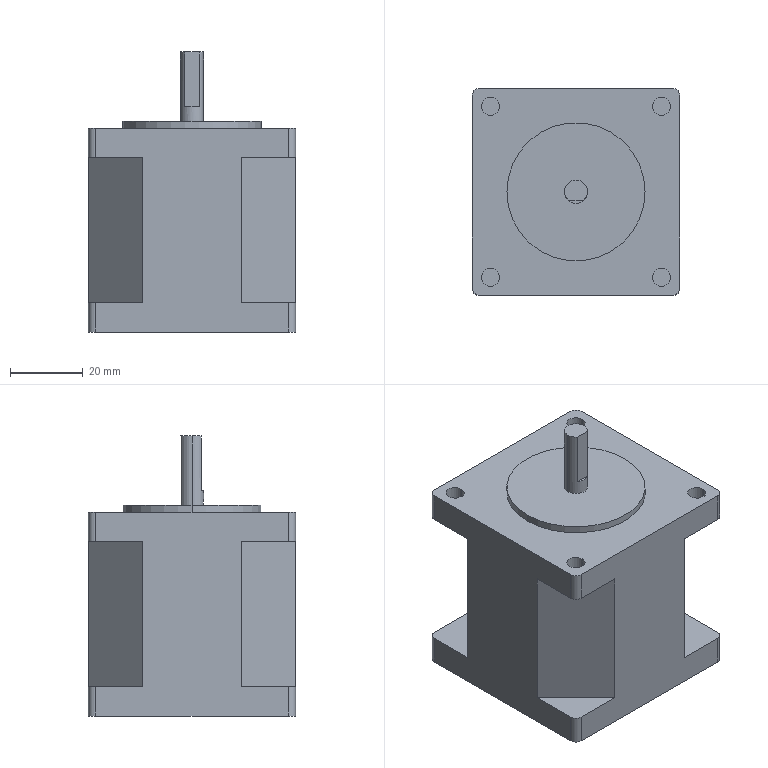Part | SolidWorks | features ICE 5, CirPattern 1, Extrusion 1, Fillet 1 | 1 solid | 42 faces | box 57 x 57 x 77 mm | volume 166104 mm3 | plane 22 | cylinder 20 | commonest cylinder face diameters 4 x8 5 x8 6.35 x2 38 x2
STEP:
#1=CARTESIAN_POINT('',(-26.,23.5,48.));
#2=VERTEX_POINT('',#1);
#3=CARTESIAN_POINT('',(-21.,23.5,48.));
#4=VERTEX_POINT('',#3);
#5=CARTESIAN_POINT('',(-23.5,23.5,48.));
#6=DIRECTION('',(0.,0.,1.));
#7=DIRECTION('',(-1.,0.,0.));
#8=AXIS2_PLACEMENT_3D('',#5,#6,#7);
#9=CIRCLE('',#8,2.5);
#10=EDGE_CURVE('',#2,#4,#9,.T.);
#11=ORIENTED_EDGE('',*,*,#10,.F.);
#12=CARTESIAN_POINT('',(-26.,23.5,56.));
#13=VERTEX_POINT('',#12);
#14=CARTESIAN_POINT('',(-26.,23.5,40.929));
#15=DIRECTION('',(0.,0.,1.));
#16=VECTOR('',#15,1000.);
#17=LINE('',#14,#16);
#18=EDGE_CURVE('',#2,#13,#17,.T.);
#19=ORIENTED_EDGE('',*,*,#18,.T.);
#20=CARTESIAN_POINT('',(-21.,23.5,56.));
#21=VERTEX_POINT('',#20);
#22=CARTESIAN_POINT('',(-23.5,23.5,56.));
#23=DIRECTION('',(0.,0.,1.));
#24=DIRECTION('',(0.,1.,0.));
#25=AXIS2_PLACEMENT_3D('',#22,#23,#24);
#26=CIRCLE('',#25,2.5);
#27=EDGE_CURVE('',#13,#21,#26,.T.);
#28=ORIENTED_EDGE('',*,*,#27,.T.);
#29=CARTESIAN_POINT('',(-21.,23.5,40.929));
#30=DIRECTION('',(0.,0.,1.));
#31=VECTOR('',#30,1000.);
#32=LINE('',#29,#31);
#33=EDGE_CURVE('',#4,#21,#32,.T.);
#34=ORIENTED_EDGE('',*,*,#33,.F.);
#35=EDGE_LOOP('',(#11,#19,#28,#34));
#36=FACE_OUTER_BOUND('',#35,.T.);
#37=CARTESIAN_POINT('',(-23.5,23.5,40.929));
#38=DIRECTION('',(0.,0.,1.));
#39=DIRECTION('',(1.,0.,0.));
#40=AXIS2_PLACEMENT_3D('',#37,#38,#39);
#41=CYLINDRICAL_SURFACE('',#40,2.5);
#42=ADVANCED_FACE('',(#36),#41,.F.);
#43=CARTESIAN_POINT('',(-26.,-23.5,48.));
#44=VERTEX_POINT('',#43);
#45=CARTESIAN_POINT('',(-21.,-23.5,48.));
#46=VERTEX_POINT('',#45);
#47=CARTESIAN_POINT('',(-23.5,-23.5,48.));
#48=DIRECTION('',(0.,0.,1.));
#49=DIRECTION('',(-1.,0.,0.));
#50=AXIS2_PLACEMENT_3D('',#47,#48,#49);
#51=CIRCLE('',#50,2.5);
#52=EDGE_CURVE('',#44,#46,#51,.T.);
#53=ORIENTED_EDGE('',*,*,#52,.F.);
#54=CARTESIAN_POINT('',(-26.,-23.5,56.));
#55=VERTEX_POINT('',#54);
#56=CARTESIAN_POINT('',(-26.,-23.5,40.929));
#57=DIRECTION('',(0.,0.,1.));
#58=VECTOR('',#57,1000.);
#59=LINE('',#56,#58);
#60=EDGE_CURVE('',#44,#55,#59,.T.);
#61=ORIENTED_EDGE('',*,*,#60,.T.);
#62=CARTESIAN_POINT('',(-21.,-23.5,56.));
#63=VERTEX_POINT('',#62);
#64=CARTESIAN_POINT('',(-23.5,-23.5,56.));
#65=DIRECTION('',(0.,0.,1.));
#66=DIRECTION('',(-1.,0.,0.));
#67=AXIS2_PLACEMENT_3D('',#64,#65,#66);
#68=CIRCLE('',#67,2.5);
#69=EDGE_CURVE('',#55,#63,#68,.T.);
#70=ORIENTED_EDGE('',*,*,#69,.T.);
#71=CARTESIAN_POINT('',(-21.,-23.5,40.929));
#72=DIRECTION('',(0.,0.,1.));
#73=VECTOR('',#72,1000.);
#74=LINE('',#71,#73);
#75=EDGE_CURVE('',#46,#63,#74,.T.);
#76=ORIENTED_EDGE('',*,*,#75,.F.);
#77=EDGE_LOOP('',(#53,#61,#70,#76));
#78=FACE_OUTER_BOUND('',#77,.T.);
#79=CARTESIAN_POINT('',(-23.5,-23.5,40.929));
#80=DIRECTION('',(0.,0.,1.));
#81=DIRECTION('',(1.,0.,0.));
#82=AXIS2_PLACEMENT_3D('',#79,#80,#81);
#83=CYLINDRICAL_SURFACE('',#82,2.5);
#84=ADVANCED_FACE('',(#78),#83,.F.);
#85=CARTESIAN_POINT('',(21.,-23.5,48.));
#86=VERTEX_POINT('',#85);
#87=CARTESIAN_POINT('',(26.,-23.5,48.));
#88=VERTEX_POINT('',#87);
#89=CARTESIAN_POINT('',(23.5,-23.5,48.));
#90=DIRECTION('',(0.,0.,1.));
#91=DIRECTION('',(-1.,0.,0.));
#92=AXIS2_PLACEMENT_3D('',#89,#90,#91);
#93=CIRCLE('',#92,2.5);
#94=EDGE_CURVE('',#86,#88,#93,.T.);
#95=ORIENTED_EDGE('',*,*,#94,.F.);
#96=CARTESIAN_POINT('',(21.,-23.5,56.));
#97=VERTEX_POINT('',#96);
#98=CARTESIAN_POINT('',(21.,-23.5,40.929));
#99=DIRECTION('',(0.,0.,1.));
#100=VECTOR('',#99,1000.);
#101=LINE('',#98,#100);
#102=EDGE_CURVE('',#86,#97,#101,.T.);
#103=ORIENTED_EDGE('',*,*,#102,.T.);
#104=CARTESIAN_POINT('',(26.,-23.5,56.));
#105=VERTEX_POINT('',#104);
#106=CARTESIAN_POINT('',(23.5,-23.5,56.));
#107=DIRECTION('',(0.,0.,1.));
#108=DIRECTION('',(0.,-1.,0.));
#109=AXIS2_PLACEMENT_3D('',#106,#107,#108);
#110=CIRCLE('',#109,2.5);
#111=EDGE_CURVE('',#97,#105,#110,.T.);
#112=ORIENTED_EDGE('',*,*,#111,.T.);
#113=CARTESIAN_POINT('',(26.,-23.5,40.929));
#114=DIRECTION('',(0.,0.,1.));
#115=VECTOR('',#114,1000.);
#116=LINE('',#113,#115);
#117=EDGE_CURVE('',#88,#105,#116,.T.);
#118=ORIENTED_EDGE('',*,*,#117,.F.);
#119=EDGE_LOOP('',(#95,#103,#112,#118));
#120=FACE_OUTER_BOUND('',#119,.T.);
#121=CARTESIAN_POINT('',(23.5,-23.5,40.929));
#122=DIRECTION('',(0.,0.,1.));
#123=DIRECTION('',(1.,0.,0.));
#124=AXIS2_PLACEMENT_3D('',#121,#122,#123);
#125=CYLINDRICAL_SURFACE('',#124,2.5);
#126=ADVANCED_FACE('',(#120),#125,.F.);
#127=CARTESIAN_POINT('',(21.,23.5,48.));
#128=VERTEX_POINT('',#127);
#129=CARTESIAN_POINT('',(26.,23.5,48.));
#130=VERTEX_POINT('',#129);
#131=CARTESIAN_POINT('',(23.5,23.5,48.));
#132=DIRECTION('',(0.,0.,1.));
#133=DIRECTION('',(-1.,0.,0.));
#134=AXIS2_PLACEMENT_3D('',#131,#132,#133);
#135=CIRCLE('',#134,2.5);
#136=EDGE_CURVE('',#128,#130,#135,.T.);
#137=ORIENTED_EDGE('',*,*,#136,.F.);
#138=CARTESIAN_POINT('',(21.,23.5,56.));
#139=VERTEX_POINT('',#138);
#140=CARTESIAN_POINT('',(21.,23.5,40.929));
#141=DIRECTION('',(0.,0.,1.));
#142=VECTOR('',#141,1000.);
#143=LINE('',#140,#142);
#144=EDGE_CURVE('',#128,#139,#143,.T.);
#145=ORIENTED_EDGE('',*,*,#144,.T.);
#146=CARTESIAN_POINT('',(26.,23.5,56.));
#147=VERTEX_POINT('',#146);
#148=CARTESIAN_POINT('',(23.5,23.5,56.));
#149=DIRECTION('',(0.,0.,1.));
#150=DIRECTION('',(1.,0.,0.));
#151=AXIS2_PLACEMENT_3D('',#148,#149,#150);
#152=CIRCLE('',#151,2.5);
#153=EDGE_CURVE('',#139,#147,#152,.T.);
#154=ORIENTED_EDGE('',*,*,#153,.T.);
#155=CARTESIAN_POINT('',(26.,23.5,40.929));
#156=DIRECTION('',(0.,0.,1.));
#157=VECTOR('',#156,1000.);
#158=LINE('',#155,#157);
#159=EDGE_CURVE('',#130,#147,#158,.T.);
#160=ORIENTED_EDGE('',*,*,#159,.F.);
#161=EDGE_LOOP('',(#137,#145,#154,#160));
#162=FACE_OUTER_BOUND('',#161,.T.);
#163=CARTESIAN_POINT('',(23.5,23.5,40.929));
#164=DIRECTION('',(0.,0.,1.));
#165=DIRECTION('',(1.,0.,0.));
#166=AXIS2_PLACEMENT_3D('',#163,#164,#165);
#167=CYLINDRICAL_SURFACE('',#166,2.5);
#168=ADVANCED_FACE('',(#162),#167,.F.);
#169=CARTESIAN_POINT('',(3.175,0.,77.));
#170=VERTEX_POINT('',#169);
#171=CARTESIAN_POINT('',(-3.175,0.,77.));
#172=VERTEX_POINT('',#171);
#173=CARTESIAN_POINT('',(0.,0.,77.));
#174=DIRECTION('',(0.,0.,1.));
#175=DIRECTION('',(1.,0.,0.));
#176=AXIS2_PLACEMENT_3D('',#173,#174,#175);
#177=CIRCLE('',#176,3.175);
#178=EDGE_CURVE('',#170,#172,#177,.T.);
#179=ORIENTED_EDGE('',*,*,#178,.F.);
#180=CARTESIAN_POINT('',(3.175,0.,58.));
#181=VERTEX_POINT('',#180);
#182=CARTESIAN_POINT('',(3.175,0.,77.));
#183=DIRECTION('',(0.,0.,-1.));
#184=VECTOR('',#183,1000.);
#185=LINE('',#182,#184);
#186=EDGE_CURVE('',#170,#181,#185,.T.);
#187=ORIENTED_EDGE('',*,*,#186,.T.);
#188=CARTESIAN_POINT('',(-3.175,0.,58.));
#189=VERTEX_POINT('',#188);
#190=CARTESIAN_POINT('',(0.,0.,58.));
#191=DIRECTION('',(0.,0.,1.));
#192=DIRECTION('',(1.,0.,0.));
#193=AXIS2_PLACEMENT_3D('',#190,#191,#192);
#194=CIRCLE('',#193,3.175);
#195=EDGE_CURVE('',#181,#189,#194,.T.);
#196=ORIENTED_EDGE('',*,*,#195,.T.);
#197=CARTESIAN_POINT('',(-3.175,0.,77.));
#198=DIRECTION('',(0.,0.,-1.));
#199=VECTOR('',#198,1000.);
#200=LINE('',#197,#199);
#201=EDGE_CURVE('',#172,#189,#200,.T.);
#202=ORIENTED_EDGE('',*,*,#201,.F.);
#203=EDGE_LOOP('',(#179,#187,#196,#202));
#204=FACE_OUTER_BOUND('',#203,.T.);
#205=CARTESIAN_POINT('',(0.,0.,77.));
#206=DIRECTION('',(0.,0.,-1.));
#207=DIRECTION('',(-1.,0.,0.));
#208=AXIS2_PLACEMENT_3D('',#205,#206,#207);
#209=CYLINDRICAL_SURFACE('',#208,3.175);
#210=ADVANCED_FACE('',(#204),#209,.T.);
#211=CARTESIAN_POINT('',(19.,0.,58.));
#212=VERTEX_POINT('',#211);
#213=CARTESIAN_POINT('',(-19.,0.,58.));
#214=VERTEX_POINT('',#213);
#215=CARTESIAN_POINT('',(0.,0.,58.));
#216=DIRECTION('',(0.,0.,1.));
#217=DIRECTION('',(1.,0.,0.));
#218=AXIS2_PLACEMENT_3D('',#215,#216,#217);
#219=CIRCLE('',#218,19.);
#220=EDGE_CURVE('',#212,#214,#219,.T.);
#221=ORIENTED_EDGE('',*,*,#220,.F.);
#222=CARTESIAN_POINT('',(19.,0.,56.));
#223=VERTEX_POINT('',#222);
#224=CARTESIAN_POINT('',(19.,0.,58.));
#225=DIRECTION('',(0.,0.,-1.));
#226=VECTOR('',#225,1000.);
#227=LINE('',#224,#226);
#228=EDGE_CURVE('',#212,#223,#227,.T.);
#229=ORIENTED_EDGE('',*,*,#228,.T.);
#230=CARTESIAN_POINT('',(-19.,0.,56.));
#231=VERTEX_POINT('',#230);
#232=CARTESIAN_POINT('',(0.,0.,56.));
#233=DIRECTION('',(0.,0.,1.));
#234=DIRECTION('',(-1.,0.,0.));
#235=AXIS2_PLACEMENT_3D('',#232,#233,#234);
#236=CIRCLE('',#235,19.);
#237=EDGE_CURVE('',#223,#231,#236,.T.);
#238=ORIENTED_EDGE('',*,*,#237,.T.);
#239=CARTESIAN_POINT('',(-19.,0.,58.));
#240=DIRECTION('',(0.,0.,-1.));
#241=VECTOR('',#240,1000.);
#242=LINE('',#239,#241);
#243=EDGE_CURVE('',#214,#231,#242,.T.);
#244=ORIENTED_EDGE('',*,*,#243,.F.);
#245=EDGE_LOOP('',(#221,#229,#238,#244));
#246=FACE_OUTER_BOUND('',#245,.T.);
#247=CARTESIAN_POINT('',(0.,0.,58.));
#248=DIRECTION('',(0.,0.,-1.));
#249=DIRECTION('',(-1.,0.,0.));
#250=AXIS2_PLACEMENT_3D('',#247,#248,#249);
#251=CYLINDRICAL_SURFACE('',#250,19.);
#252=ADVANCED_FACE('',(#246),#251,.T.);
#253=CARTESIAN_POINT('',(28.5,-26.5,8.));
#254=VERTEX_POINT('',#253);
#255=CARTESIAN_POINT('',(28.5,-13.5,8.));
#256=VERTEX_POINT('',#255);
#257=CARTESIAN_POINT('',(28.5,-28.5,8.));
#258=DIRECTION('',(0.,1.,0.));
#259=VECTOR('',#258,1000.);
#260=LINE('',#257,#259);
#261=EDGE_CURVE('',#254,#256,#260,.T.);
#262=ORIENTED_EDGE('',*,*,#261,.F.);
#263=CARTESIAN_POINT('',(28.5,-26.5,0.));
#264=VERTEX_POINT('',#263);
#265=CARTESIAN_POINT('',(28.5,-26.5,56.));
#266=DIRECTION('',(0.,0.,-1.));
#267=VECTOR('',#266,1000.);
#268=LINE('',#265,#267);
#269=EDGE_CURVE('',#254,#264,#268,.T.);
#270=ORIENTED_EDGE('',*,*,#269,.T.);
#271=CARTESIAN_POINT('',(28.5,26.5,0.));
#272=VERTEX_POINT('',#271);
#273=CARTESIAN_POINT('',(28.5,-28.5,0.));
#274=DIRECTION('',(0.,1.,0.));
#275=VECTOR('',#274,1000.);
#276=LINE('',#273,#275);
#277=EDGE_CURVE('',#264,#272,#276,.T.);
#278=ORIENTED_EDGE('',*,*,#277,.T.);
#279=CARTESIAN_POINT('',(28.5,26.5,8.));
#280=VERTEX_POINT('',#279);
#281=CARTESIAN_POINT('',(28.5,26.5,56.));
#282=DIRECTION('',(0.,0.,1.));
#283=VECTOR('',#282,1000.);
#284=LINE('',#281,#283);
#285=EDGE_CURVE('',#272,#280,#284,.T.);
#286=ORIENTED_EDGE('',*,*,#285,.T.);
#287=CARTESIAN_POINT('',(28.5,13.5,8.));
#288=VERTEX_POINT('',#287);
#289=CARTESIAN_POINT('',(28.5,13.5,8.));
#290=DIRECTION('',(0.,1.,0.));
#291=VECTOR('',#290,1000.);
#292=LINE('',#289,#291);
#293=EDGE_CURVE('',#288,#280,#292,.T.);
#294=ORIENTED_EDGE('',*,*,#293,.F.);
#295=CARTESIAN_POINT('',(28.5,13.5,48.));
#296=VERTEX_POINT('',#295);
#297=CARTESIAN_POINT('',(28.5,13.5,8.));
#298=DIRECTION('',(0.,0.,1.));
#299=VECTOR('',#298,1000.);
#300=LINE('',#297,#299);
#301=EDGE_CURVE('',#288,#296,#300,.T.);
#302=ORIENTED_EDGE('',*,*,#301,.T.);
#303=CARTESIAN_POINT('',(28.5,26.5,48.));
#304=VERTEX_POINT('',#303);
#305=CARTESIAN_POINT('',(28.5,13.5,48.));
#306=DIRECTION('',(0.,1.,0.));
#307=VECTOR('',#306,1000.);
#308=LINE('',#305,#307);
#309=EDGE_CURVE('',#296,#304,#308,.T.);
#310=ORIENTED_EDGE('',*,*,#309,.T.);
#311=CARTESIAN_POINT('',(28.5,26.5,56.));
#312=VERTEX_POINT('',#311);
#313=CARTESIAN_POINT('',(28.5,26.5,56.));
#314=DIRECTION('',(0.,0.,1.));
#315=VECTOR('',#314,1000.);
#316=LINE('',#313,#315);
#317=EDGE_CURVE('',#304,#312,#316,.T.);
#318=ORIENTED_EDGE('',*,*,#317,.T.);
#319=CARTESIAN_POINT('',(28.5,-26.5,56.));
#320=VERTEX_POINT('',#319);
#321=CARTESIAN_POINT('',(28.5,-28.5,56.));
#322=DIRECTION('',(0.,1.,0.));
#323=VECTOR('',#322,1000.);
#324=LINE('',#321,#323);
#325=EDGE_CURVE('',#320,#312,#324,.T.);
#326=ORIENTED_EDGE('',*,*,#325,.F.);
#327=CARTESIAN_POINT('',(28.5,-26.5,48.));
#328=VERTEX_POINT('',#327);
#329=CARTESIAN_POINT('',(28.5,-26.5,56.));
#330=DIRECTION('',(0.,0.,-1.));
#331=VECTOR('',#330,1000.);
#332=LINE('',#329,#331);
#333=EDGE_CURVE('',#320,#328,#332,.T.);
#334=ORIENTED_EDGE('',*,*,#333,.T.);
#335=CARTESIAN_POINT('',(28.5,-13.5,48.));
#336=VERTEX_POINT('',#335);
#337=CARTESIAN_POINT('',(28.5,-28.5,48.));
#338=DIRECTION('',(0.,1.,0.));
#339=VECTOR('',#338,1000.);
#340=LINE('',#337,#339);
#341=EDGE_CURVE('',#328,#336,#340,.T.);
#342=ORIENTED_EDGE('',*,*,#341,.T.);
#343=CARTESIAN_POINT('',(28.5,-13.5,8.));
#344=DIRECTION('',(0.,0.,1.));
#345=VECTOR('',#344,1000.);
#346=LINE('',#343,#345);
#347=EDGE_CURVE('',#256,#336,#346,.T.);
#348=ORIENTED_EDGE('',*,*,#347,.F.);
#349=EDGE_LOOP('',(#262,#270,#278,#286,#294,#302,#310,#318,#326,#334,#342,#348));
#350=FACE_OUTER_BOUND('',#349,.T.);
#351=CARTESIAN_POINT('',(28.5,-28.5,56.));
#352=DIRECTION('',(-1.,0.,0.));
#353=DIRECTION('',(0.,0.,1.));
#354=AXIS2_PLACEMENT_3D('',#351,#352,#353);
#355=PLANE('',#354);
#356=ADVANCED_FACE('',(#350),#355,.F.);
#357=CARTESIAN_POINT('',(26.5,28.5,0.));
#358=VERTEX_POINT('',#357);
#359=CARTESIAN_POINT('',(-26.5,28.5,0.));
#360=VERTEX_POINT('',#359);
#361=CARTESIAN_POINT('',(-28.5,28.5,0.));
#362=DIRECTION('',(-1.,0.,0.));
#363=VECTOR('',#362,1000.);
#364=LINE('',#361,#363);
#365=EDGE_CURVE('',#358,#360,#364,.T.);
#366=ORIENTED_EDGE('',*,*,#365,.T.);
#367=CARTESIAN_POINT('',(-26.5,28.5,8.));
#368=VERTEX_POINT('',#367);
#369=CARTESIAN_POINT('',(-26.5,28.5,56.));
#370=DIRECTION('',(0.,0.,1.));
#371=VECTOR('',#370,1000.);
#372=LINE('',#369,#371);
#373=EDGE_CURVE('',#360,#368,#372,.T.);
#374=ORIENTED_EDGE('',*,*,#373,.T.);
#375=CARTESIAN_POINT('',(-13.5,28.5,8.));
#376=VERTEX_POINT('',#375);
#377=CARTESIAN_POINT('',(-13.5,28.5,8.));
#378=DIRECTION('',(-1.,0.,0.));
#379=VECTOR('',#378,1000.);
#380=LINE('',#377,#379);
#381=EDGE_CURVE('',#376,#368,#380,.T.);
#382=ORIENTED_EDGE('',*,*,#381,.F.);
#383=CARTESIAN_POINT('',(-13.5,28.5,48.));
#384=VERTEX_POINT('',#383);
#385=CARTESIAN_POINT('',(-13.5,28.5,8.));
#386=DIRECTION('',(0.,0.,1.));
#387=VECTOR('',#386,1000.);
#388=LINE('',#385,#387);
#389=EDGE_CURVE('',#376,#384,#388,.T.);
#390=ORIENTED_EDGE('',*,*,#389,.T.);
#391=CARTESIAN_POINT('',(-26.5,28.5,48.));
#392=VERTEX_POINT('',#391);
#393=CARTESIAN_POINT('',(-13.5,28.5,48.));
#394=DIRECTION('',(-1.,0.,0.));
#395=VECTOR('',#394,1000.);
#396=LINE('',#393,#395);
#397=EDGE_CURVE('',#384,#392,#396,.T.);
#398=ORIENTED_EDGE('',*,*,#397,.T.);
#399=CARTESIAN_POINT('',(-26.5,28.5,56.));
#400=VERTEX_POINT('',#399);
#401=CARTESIAN_POINT('',(-26.5,28.5,56.));
#402=DIRECTION('',(0.,0.,1.));
#403=VECTOR('',#402,1000.);
#404=LINE('',#401,#403);
#405=EDGE_CURVE('',#392,#400,#404,.T.);
#406=ORIENTED_EDGE('',*,*,#405,.T.);
#407=CARTESIAN_POINT('',(26.5,28.5,56.));
#408=VERTEX_POINT('',#407);
#409=CARTESIAN_POINT('',(-28.5,28.5,56.));
#410=DIRECTION('',(-1.,0.,0.));
#411=VECTOR('',#410,1000.);
#412=LINE('',#409,#411);
#413=EDGE_CURVE('',#408,#400,#412,.T.);
#414=ORIENTED_EDGE('',*,*,#413,.F.);
#415=CARTESIAN_POINT('',(26.5,28.5,48.));
#416=VERTEX_POINT('',#415);
#417=CARTESIAN_POINT('',(26.5,28.5,56.));
#418=DIRECTION('',(0.,0.,-1.));
#419=VECTOR('',#418,1000.);
#420=LINE('',#417,#419);
#421=EDGE_CURVE('',#408,#416,#420,.T.);
#422=ORIENTED_EDGE('',*,*,#421,.T.);
#423=CARTESIAN_POINT('',(13.5,28.5,48.));
#424=VERTEX_POINT('',#423);
#425=CARTESIAN_POINT('',(28.5,28.5,48.));
#426=DIRECTION('',(-1.,0.,0.));
#427=VECTOR('',#426,1000.);
#428=LINE('',#425,#427);
#429=EDGE_CURVE('',#416,#424,#428,.T.);
#430=ORIENTED_EDGE('',*,*,#429,.T.);
#431=CARTESIAN_POINT('',(13.5,28.5,8.));
#432=VERTEX_POINT('',#431);
#433=CARTESIAN_POINT('',(13.5,28.5,8.));
#434=DIRECTION('',(0.,0.,1.));
#435=VECTOR('',#434,1000.);
#436=LINE('',#433,#435);
#437=EDGE_CURVE('',#432,#424,#436,.T.);
#438=ORIENTED_EDGE('',*,*,#437,.F.);
#439=CARTESIAN_POINT('',(26.5,28.5,8.));
#440=VERTEX_POINT('',#439);
#441=CARTESIAN_POINT('',(28.5,28.5,8.));
#442=DIRECTION('',(-1.,0.,0.));
#443=VECTOR('',#442,1000.);
#444=LINE('',#441,#443);
#445=EDGE_CURVE('',#440,#432,#444,.T.);
#446=ORIENTED_EDGE('',*,*,#445,.F.);
#447=CARTESIAN_POINT('',(26.5,28.5,56.));
#448=DIRECTION('',(0.,0.,-1.));
#449=VECTOR('',#448,1000.);
#450=LINE('',#447,#449);
#451=EDGE_CURVE('',#440,#358,#450,.T.);
#452=ORIENTED_EDGE('',*,*,#451,.T.);
#453=EDGE_LOOP('',(#366,#374,#382,#390,#398,#406,#414,#422,#430,#438,#446,#452));
#454=FACE_OUTER_BOUND('',#453,.T.);
#455=CARTESIAN_POINT('',(-28.5,28.5,56.));
#456=DIRECTION('',(0.,-1.,0.));
#457=DIRECTION('',(0.,0.,-1.));
#458=AXIS2_PLACEMENT_3D('',#455,#456,#457);
#459=PLANE('',#458);
#460=ADVANCED_FACE('',(#454),#459,.F.);
#461=CARTESIAN_POINT('',(-28.5,26.5,8.));
#462=VERTEX_POINT('',#461);
#463=CARTESIAN_POINT('',(-28.5,13.5,8.));
#464=VERTEX_POINT('',#463);
#465=CARTESIAN_POINT('',(-28.5,28.5,8.));
#466=DIRECTION('',(0.,-1.,0.));
#467=VECTOR('',#466,1000.);
#468=LINE('',#465,#467);
#469=EDGE_CURVE('',#462,#464,#468,.T.);
#470=ORIENTED_EDGE('',*,*,#469,.F.);
#471=CARTESIAN_POINT('',(-28.5,26.5,0.));
#472=VERTEX_POINT('',#471);
#473=CARTESIAN_POINT('',(-28.5,26.5,56.));
#474=DIRECTION('',(0.,0.,-1.));
#475=VECTOR('',#474,1000.);
#476=LINE('',#473,#475);
#477=EDGE_CURVE('',#462,#472,#476,.T.);
#478=ORIENTED_EDGE('',*,*,#477,.T.);
#479=CARTESIAN_POINT('',(-28.5,-26.5,0.));
#480=VERTEX_POINT('',#479);
#481=CARTESIAN_POINT('',(-28.5,-28.5,0.));
#482=DIRECTION('',(0.,-1.,0.));
#483=VECTOR('',#482,1000.);
#484=LINE('',#481,#483);
#485=EDGE_CURVE('',#472,#480,#484,.T.);
#486=ORIENTED_EDGE('',*,*,#485,.T.);
#487=CARTESIAN_POINT('',(-28.5,-26.5,8.));
#488=VERTEX_POINT('',#487);
#489=CARTESIAN_POINT('',(-28.5,-26.5,56.));
#490=DIRECTION('',(0.,0.,1.));
#491=VECTOR('',#490,1000.);
#492=LINE('',#489,#491);
#493=EDGE_CURVE('',#480,#488,#492,.T.);
#494=ORIENTED_EDGE('',*,*,#493,.T.);
#495=CARTESIAN_POINT('',(-28.5,-13.5,8.));
#496=VERTEX_POINT('',#495);
#497=CARTESIAN_POINT('',(-28.5,-13.5,8.));
#498=DIRECTION('',(0.,-1.,0.));
#499=VECTOR('',#498,1000.);
#500=LINE('',#497,#499);
#501=EDGE_CURVE('',#496,#488,#500,.T.);
#502=ORIENTED_EDGE('',*,*,#501,.F.);
#503=CARTESIAN_POINT('',(-28.5,-13.5,48.));
#504=VERTEX_POINT('',#503);
#505=CARTESIAN_POINT('',(-28.5,-13.5,8.));
#506=DIRECTION('',(0.,0.,1.));
#507=VECTOR('',#506,1000.);
#508=LINE('',#505,#507);
#509=EDGE_CURVE('',#496,#504,#508,.T.);
#510=ORIENTED_EDGE('',*,*,#509,.T.);
#511=CARTESIAN_POINT('',(-28.5,-26.5,48.));
#512=VERTEX_POINT('',#511);
#513=CARTESIAN_POINT('',(-28.5,-13.5,48.));
#514=DIRECTION('',(0.,-1.,0.));
#515=VECTOR('',#514,1000.);
#516=LINE('',#513,#515);
#517=EDGE_CURVE('',#504,#512,#516,.T.);
#518=ORIENTED_EDGE('',*,*,#517,.T.);
#519=CARTESIAN_POINT('',(-28.5,-26.5,56.));
#520=VERTEX_POINT('',#519);
#521=CARTESIAN_POINT('',(-28.5,-26.5,56.));
#522=DIRECTION('',(0.,0.,1.));
#523=VECTOR('',#522,1000.);
#524=LINE('',#521,#523);
#525=EDGE_CURVE('',#512,#520,#524,.T.);
#526=ORIENTED_EDGE('',*,*,#525,.T.);
#527=CARTESIAN_POINT('',(-28.5,26.5,56.));
#528=VERTEX_POINT('',#527);
#529=CARTESIAN_POINT('',(-28.5,-28.5,56.));
#530=DIRECTION('',(0.,-1.,0.));
#531=VECTOR('',#530,1000.);
#532=LINE('',#529,#531);
#533=EDGE_CURVE('',#528,#520,#532,.T.);
#534=ORIENTED_EDGE('',*,*,#533,.F.);
#535=CARTESIAN_POINT('',(-28.5,26.5,48.));
#536=VERTEX_POINT('',#535);
#537=CARTESIAN_POINT('',(-28.5,26.5,56.));
#538=DIRECTION('',(0.,0.,-1.));
#539=VECTOR('',#538,1000.);
#540=LINE('',#537,#539);
#541=EDGE_CURVE('',#528,#536,#540,.T.);
#542=ORIENTED_EDGE('',*,*,#541,.T.);
#543=CARTESIAN_POINT('',(-28.5,13.5,48.));
#544=VERTEX_POINT('',#543);
#545=CARTESIAN_POINT('',(-28.5,28.5,48.));
#546=DIRECTION('',(0.,-1.,0.));
#547=VECTOR('',#546,1000.);
#548=LINE('',#545,#547);
#549=EDGE_CURVE('',#536,#544,#548,.T.);
#550=ORIENTED_EDGE('',*,*,#549,.T.);
#551=CARTESIAN_POINT('',(-28.5,13.5,8.));
#552=DIRECTION('',(0.,0.,1.));
#553=VECTOR('',#552,1000.);
#554=LINE('',#551,#553);
#555=EDGE_CURVE('',#464,#544,#554,.T.);
#556=ORIENTED_EDGE('',*,*,#555,.F.);
#557=EDGE_LOOP('',(#470,#478,#486,#494,#502,#510,#518,#526,#534,#542,#550,#556));
#558=FACE_OUTER_BOUND('',#557,.T.);
#559=CARTESIAN_POINT('',(-28.5,-28.5,56.));
#560=DIRECTION('',(1.,0.,0.));
#561=DIRECTION('',(0.,0.,-1.));
#562=AXIS2_PLACEMENT_3D('',#559,#560,#561);
#563=PLANE('',#562);
#564=ADVANCED_FACE('',(#558),#563,.F.);
#565=CARTESIAN_POINT('',(-26.5,-28.5,8.));
#566=VERTEX_POINT('',#565);
#567=CARTESIAN_POINT('',(-13.5,-28.5,8.));
#568=VERTEX_POINT('',#567);
#569=CARTESIAN_POINT('',(-28.5,-28.5,8.));
#570=DIRECTION('',(1.,0.,0.));
#571=VECTOR('',#570,1000.);
#572=LINE('',#569,#571);
#573=EDGE_CURVE('',#566,#568,#572,.T.);
#574=ORIENTED_EDGE('',*,*,#573,.F.);
#575=CARTESIAN_POINT('',(-26.5,-28.5,0.));
#576=VERTEX_POINT('',#575);
#577=CARTESIAN_POINT('',(-26.5,-28.5,56.));
#578=DIRECTION('',(0.,0.,-1.));
#579=VECTOR('',#578,1000.);
#580=LINE('',#577,#579);
#581=EDGE_CURVE('',#566,#576,#580,.T.);
#582=ORIENTED_EDGE('',*,*,#581,.T.);
#583=CARTESIAN_POINT('',(26.5,-28.5,0.));
#584=VERTEX_POINT('',#583);
#585=CARTESIAN_POINT('',(-28.5,-28.5,0.));
#586=DIRECTION('',(1.,0.,0.));
#587=VECTOR('',#586,1000.);
#588=LINE('',#585,#587);
#589=EDGE_CURVE('',#576,#584,#588,.T.);
#590=ORIENTED_EDGE('',*,*,#589,.T.);
#591=CARTESIAN_POINT('',(26.5,-28.5,8.));
#592=VERTEX_POINT('',#591);
#593=CARTESIAN_POINT('',(26.5,-28.5,56.));
#594=DIRECTION('',(0.,0.,1.));
#595=VECTOR('',#594,1000.);
#596=LINE('',#593,#595);
#597=EDGE_CURVE('',#584,#592,#596,.T.);
#598=ORIENTED_EDGE('',*,*,#597,.T.);
#599=CARTESIAN_POINT('',(13.5,-28.5,8.));
#600=VERTEX_POINT('',#599);
#601=CARTESIAN_POINT('',(13.5,-28.5,8.));
#602=DIRECTION('',(1.,0.,0.));
#603=VECTOR('',#602,1000.);
#604=LINE('',#601,#603);
#605=EDGE_CURVE('',#600,#592,#604,.T.);
#606=ORIENTED_EDGE('',*,*,#605,.F.);
#607=CARTESIAN_POINT('',(13.5,-28.5,48.));
#608=VERTEX_POINT('',#607);
#609=CARTESIAN_POINT('',(13.5,-28.5,8.));
#610=DIRECTION('',(0.,0.,1.));
#611=VECTOR('',#610,1000.);
#612=LINE('',#609,#611);
#613=EDGE_CURVE('',#600,#608,#612,.T.);
#614=ORIENTED_EDGE('',*,*,#613,.T.);
#615=CARTESIAN_POINT('',(26.5,-28.5,48.));
#616=VERTEX_POINT('',#615);
#617=CARTESIAN_POINT('',(13.5,-28.5,48.));
#618=DIRECTION('',(1.,0.,0.));
#619=VECTOR('',#618,1000.);
#620=LINE('',#617,#619);
#621=EDGE_CURVE('',#608,#616,#620,.T.);
#622=ORIENTED_EDGE('',*,*,#621,.T.);
#623=CARTESIAN_POINT('',(26.5,-28.5,56.));
#624=VERTEX_POINT('',#623);
#625=CARTESIAN_POINT('',(26.5,-28.5,56.));
#626=DIRECTION('',(0.,0.,1.));
#627=VECTOR('',#626,1000.);
#628=LINE('',#625,#627);
#629=EDGE_CURVE('',#616,#624,#628,.T.);
#630=ORIENTED_EDGE('',*,*,#629,.T.);
#631=CARTESIAN_POINT('',(-26.5,-28.5,56.));
#632=VERTEX_POINT('',#631);
#633=CARTESIAN_POINT('',(-28.5,-28.5,56.));
#634=DIRECTION('',(1.,0.,0.));
#635=VECTOR('',#634,1000.);
#636=LINE('',#633,#635);
#637=EDGE_CURVE('',#632,#624,#636,.T.);
#638=ORIENTED_EDGE('',*,*,#637,.F.);
#639=CARTESIAN_POINT('',(-26.5,-28.5,48.));
#640=VERTEX_POINT('',#639);
#641=CARTESIAN_POINT('',(-26.5,-28.5,56.));
#642=DIRECTION('',(0.,0.,-1.));
#643=VECTOR('',#642,1000.);
#644=LINE('',#641,#643);
#645=EDGE_CURVE('',#632,#640,#644,.T.);
#646=ORIENTED_EDGE('',*,*,#645,.T.);
#647=CARTESIAN_POINT('',(-13.5,-28.5,48.));
#648=VERTEX_POINT('',#647);
#649=CARTESIAN_POINT('',(-28.5,-28.5,48.));
#650=DIRECTION('',(1.,0.,0.));
#651=VECTOR('',#650,1000.);
#652=LINE('',#649,#651);
#653=EDGE_CURVE('',#640,#648,#652,.T.);
#654=ORIENTED_EDGE('',*,*,#653,.T.);
#655=CARTESIAN_POINT('',(-13.5,-28.5,8.));
#656=DIRECTION('',(0.,0.,1.));
#657=VECTOR('',#656,1000.);
#658=LINE('',#655,#657);
#659=EDGE_CURVE('',#568,#648,#658,.T.);
#660=ORIENTED_EDGE('',*,*,#659,.F.);
#661=EDGE_LOOP('',(#574,#582,#590,#598,#606,#614,#622,#630,#638,#646,#654,#660));
#662=FACE_OUTER_BOUND('',#661,.T.);
#663=CARTESIAN_POINT('',(-28.5,-28.5,56.));
#664=DIRECTION('',(0.,1.,0.));
#665=DIRECTION('',(0.,0.,1.));
#666=AXIS2_PLACEMENT_3D('',#663,#664,#665);
#667=PLANE('',#666);
#668=ADVANCED_FACE('',(#662),#667,.F.);
#669=CARTESIAN_POINT('',(-23.5,23.5,56.));
#670=DIRECTION('',(0.,0.,1.));
#671=DIRECTION('',(0.,1.,0.));
#672=AXIS2_PLACEMENT_3D('',#669,#670,#671);
#673=CIRCLE('',#672,2.5);
#674=EDGE_CURVE('',#21,#13,#673,.T.);
#675=ORIENTED_EDGE('',*,*,#674,.F.);
#676=ORIENTED_EDGE('',*,*,#27,.F.);
#677=EDGE_LOOP('',(#675,#676));
#678=FACE_BOUND('',#677,.T.);
#679=CARTESIAN_POINT('',(-23.5,-23.5,56.));
#680=DIRECTION('',(0.,0.,1.));
#681=DIRECTION('',(-1.,0.,0.));
#682=AXIS2_PLACEMENT_3D('',#679,#680,#681);
#683=CIRCLE('',#682,2.5);
#684=EDGE_CURVE('',#63,#55,#683,.T.);
#685=ORIENTED_EDGE('',*,*,#684,.F.);
#686=ORIENTED_EDGE('',*,*,#69,.F.);
#687=EDGE_LOOP('',(#685,#686));
#688=FACE_BOUND('',#687,.T.);
#689=CARTESIAN_POINT('',(23.5,-23.5,56.));
#690=DIRECTION('',(0.,0.,1.));
#691=DIRECTION('',(0.,-1.,0.));
#692=AXIS2_PLACEMENT_3D('',#689,#690,#691);
#693=CIRCLE('',#692,2.5);
#694=EDGE_CURVE('',#105,#97,#693,.T.);
#695=ORIENTED_EDGE('',*,*,#694,.F.);
#696=ORIENTED_EDGE('',*,*,#111,.F.);
#697=EDGE_LOOP('',(#695,#696));
#698=FACE_BOUND('',#697,.T.);
#699=CARTESIAN_POINT('',(23.5,23.5,56.));
#700=DIRECTION('',(0.,0.,1.));
#701=DIRECTION('',(1.,0.,0.));
#702=AXIS2_PLACEMENT_3D('',#699,#700,#701);
#703=CIRCLE('',#702,2.5);
#704=EDGE_CURVE('',#147,#139,#703,.T.);
#705=ORIENTED_EDGE('',*,*,#704,.F.);
#706=ORIENTED_EDGE('',*,*,#153,.F.);
#707=EDGE_LOOP('',(#705,#706));
#708=FACE_BOUND('',#707,.T.);
#709=CARTESIAN_POINT('',(0.,0.,56.));
#710=DIRECTION('',(0.,0.,1.));
#711=DIRECTION('',(-1.,0.,0.));
#712=AXIS2_PLACEMENT_3D('',#709,#710,#711);
#713=CIRCLE('',#712,19.);
#714=EDGE_CURVE('',#231,#223,#713,.T.);
#715=ORIENTED_EDGE('',*,*,#714,.F.);
#716=ORIENTED_EDGE('',*,*,#237,.F.);
#717=EDGE_LOOP('',(#715,#716));
#718=FACE_BOUND('',#717,.T.);
#719=ORIENTED_EDGE('',*,*,#413,.T.);
#720=CARTESIAN_POINT('',(-26.5,26.5,56.));
#721=DIRECTION('',(0.,0.,1.));
#722=DIRECTION('',(-1.,0.,0.));
#723=AXIS2_PLACEMENT_3D('',#720,#721,#722);
#724=CIRCLE('',#723,2.);
#725=EDGE_CURVE('',#400,#528,#724,.T.);
#726=ORIENTED_EDGE('',*,*,#725,.T.);
#727=ORIENTED_EDGE('',*,*,#533,.T.);
#728=CARTESIAN_POINT('',(-26.5,-26.5,56.));
#729=DIRECTION('',(0.,0.,1.));
#730=DIRECTION('',(-1.,0.,0.));
#731=AXIS2_PLACEMENT_3D('',#728,#729,#730);
#732=CIRCLE('',#731,2.);
#733=EDGE_CURVE('',#520,#632,#732,.T.);
#734=ORIENTED_EDGE('',*,*,#733,.T.);
#735=ORIENTED_EDGE('',*,*,#637,.T.);
#736=CARTESIAN_POINT('',(26.5,-26.5,56.));
#737=DIRECTION('',(0.,0.,1.));
#738=DIRECTION('',(-1.,0.,0.));
#739=AXIS2_PLACEMENT_3D('',#736,#737,#738);
#740=CIRCLE('',#739,2.);
#741=EDGE_CURVE('',#624,#320,#740,.T.);
#742=ORIENTED_EDGE('',*,*,#741,.T.);
#743=ORIENTED_EDGE('',*,*,#325,.T.);
#744=CARTESIAN_POINT('',(26.5,26.5,56.));
#745=DIRECTION('',(0.,0.,1.));
#746=DIRECTION('',(-1.,0.,0.));
#747=AXIS2_PLACEMENT_3D('',#744,#745,#746);
#748=CIRCLE('',#747,2.);
#749=EDGE_CURVE('',#312,#408,#748,.T.);
#750=ORIENTED_EDGE('',*,*,#749,.T.);
#751=EDGE_LOOP('',(#719,#726,#727,#734,#735,#742,#743,#750));
#752=FACE_OUTER_BOUND('',#751,.T.);
#753=CARTESIAN_POINT('',(0.,0.,56.));
#754=DIRECTION('',(0.,0.,-1.));
#755=DIRECTION('',(-1.,0.,0.));
#756=AXIS2_PLACEMENT_3D('',#753,#754,#755);
#757=PLANE('',#756);
#758=ADVANCED_FACE('',(#678,#688,#698,#708,#718,#752),#757,.F.);
#759=ORIENTED_EDGE('',*,*,#485,.F.);
#760=CARTESIAN_POINT('',(-26.5,26.5,0.));
#761=DIRECTION('',(0.,0.,-1.));
#762=DIRECTION('',(-1.,0.,0.));
#763=AXIS2_PLACEMENT_3D('',#760,#761,#762);
#764=CIRCLE('',#763,2.);
#765=EDGE_CURVE('',#472,#360,#764,.T.);
#766=ORIENTED_EDGE('',*,*,#765,.T.);
#767=ORIENTED_EDGE('',*,*,#365,.F.);
#768=CARTESIAN_POINT('',(26.5,26.5,0.));
#769=DIRECTION('',(0.,0.,-1.));
#770=DIRECTION('',(-1.,0.,0.));
#771=AXIS2_PLACEMENT_3D('',#768,#769,#770);
#772=CIRCLE('',#771,2.);
#773=EDGE_CURVE('',#358,#272,#772,.T.);
#774=ORIENTED_EDGE('',*,*,#773,.T.);
#775=ORIENTED_EDGE('',*,*,#277,.F.);
#776=CARTESIAN_POINT('',(26.5,-26.5,0.));
#777=DIRECTION('',(0.,0.,-1.));
#778=DIRECTION('',(-1.,0.,0.));
#779=AXIS2_PLACEMENT_3D('',#776,#777,#778);
#780=CIRCLE('',#779,2.);
#781=EDGE_CURVE('',#264,#584,#780,.T.);
#782=ORIENTED_EDGE('',*,*,#781,.T.);
#783=ORIENTED_EDGE('',*,*,#589,.F.);
#784=CARTESIAN_POINT('',(-26.5,-26.5,0.));
#785=DIRECTION('',(0.,0.,-1.));
#786=DIRECTION('',(-1.,0.,0.));
#787=AXIS2_PLACEMENT_3D('',#784,#785,#786);
#788=CIRCLE('',#787,2.);
#789=EDGE_CURVE('',#576,#480,#788,.T.);
#790=ORIENTED_EDGE('',*,*,#789,.T.);
#791=EDGE_LOOP('',(#759,#766,#767,#774,#775,#782,#783,#790));
#792=FACE_OUTER_BOUND('',#791,.T.);
#793=CARTESIAN_POINT('',(0.,0.,0.));
#794=DIRECTION('',(0.,0.,-1.));
#795=DIRECTION('',(-1.,0.,0.));
#796=AXIS2_PLACEMENT_3D('',#793,#794,#795);
#797=PLANE('',#796);
#798=ADVANCED_FACE('',(#792),#797,.T.);
#799=ORIENTED_EDGE('',*,*,#228,.F.);
#800=CARTESIAN_POINT('',(0.,0.,58.));
#801=DIRECTION('',(0.,0.,1.));
#802=DIRECTION('',(1.,0.,0.));
#803=AXIS2_PLACEMENT_3D('',#800,#801,#802);
#804=CIRCLE('',#803,19.);
#805=EDGE_CURVE('',#214,#212,#804,.T.);
#806=ORIENTED_EDGE('',*,*,#805,.F.);
#807=ORIENTED_EDGE('',*,*,#243,.T.);
#808=ORIENTED_EDGE('',*,*,#714,.T.);
#809=EDGE_LOOP('',(#799,#806,#807,#808));
#810=FACE_OUTER_BOUND('',#809,.T.);
#811=CARTESIAN_POINT('',(0.,0.,58.));
#812=DIRECTION('',(0.,0.,-1.));
#813=DIRECTION('',(-1.,0.,0.));
#814=AXIS2_PLACEMENT_3D('',#811,#812,#813);
#815=CYLINDRICAL_SURFACE('',#814,19.);
#816=ADVANCED_FACE('',(#810),#815,.T.);
#817=CARTESIAN_POINT('',(0.,0.,58.));
#818=DIRECTION('',(0.,0.,1.));
#819=DIRECTION('',(1.,0.,0.));
#820=AXIS2_PLACEMENT_3D('',#817,#818,#819);
#821=CIRCLE('',#820,3.175);
#822=EDGE_CURVE('',#189,#181,#821,.T.);
#823=ORIENTED_EDGE('',*,*,#822,.F.);
#824=ORIENTED_EDGE('',*,*,#195,.F.);
#825=EDGE_LOOP('',(#823,#824));
#826=FACE_BOUND('',#825,.T.);
#827=ORIENTED_EDGE('',*,*,#805,.T.);
#828=ORIENTED_EDGE('',*,*,#220,.T.);
#829=EDGE_LOOP('',(#827,#828));
#830=FACE_OUTER_BOUND('',#829,.T.);
#831=CARTESIAN_POINT('',(0.,0.,58.));
#832=DIRECTION('',(0.,0.,1.));
#833=DIRECTION('',(1.,0.,0.));
#834=AXIS2_PLACEMENT_3D('',#831,#832,#833);
#835=PLANE('',#834);
#836=ADVANCED_FACE('',(#826,#830),#835,.T.);
#837=ORIENTED_EDGE('',*,*,#186,.F.);
#838=CARTESIAN_POINT('',(1.957,-2.5,77.));
#839=VERTEX_POINT('',#838);
#840=CARTESIAN_POINT('',(0.,0.,77.));
#841=DIRECTION('',(0.,0.,1.));
#842=DIRECTION('',(1.,0.,0.));
#843=AXIS2_PLACEMENT_3D('',#840,#841,#842);
#844=CIRCLE('',#843,3.175);
#845=EDGE_CURVE('',#839,#170,#844,.T.);
#846=ORIENTED_EDGE('',*,*,#845,.F.);
#847=CARTESIAN_POINT('',(1.957,-2.5,62.));
#848=VERTEX_POINT('',#847);
#849=CARTESIAN_POINT('',(1.957,-2.5,77.));
#850=DIRECTION('',(0.,0.,-1.));
#851=VECTOR('',#850,1000.);
#852=LINE('',#849,#851);
#853=EDGE_CURVE('',#839,#848,#852,.T.);
#854=ORIENTED_EDGE('',*,*,#853,.T.);
#855=CARTESIAN_POINT('',(-1.957,-2.5,62.));
#856=VERTEX_POINT('',#855);
#857=CARTESIAN_POINT('',(0.,0.,62.));
#858=DIRECTION('',(0.,0.,1.));
#859=DIRECTION('',(1.,0.,0.));
#860=AXIS2_PLACEMENT_3D('',#857,#858,#859);
#861=CIRCLE('',#860,3.175);
#862=EDGE_CURVE('',#856,#848,#861,.T.);
#863=ORIENTED_EDGE('',*,*,#862,.F.);
#864=CARTESIAN_POINT('',(-1.957,-2.5,77.));
#865=VERTEX_POINT('',#864);
#866=CARTESIAN_POINT('',(-1.957,-2.5,77.));
#867=DIRECTION('',(0.,0.,1.));
#868=VECTOR('',#867,1000.);
#869=LINE('',#866,#868);
#870=EDGE_CURVE('',#856,#865,#869,.T.);
#871=ORIENTED_EDGE('',*,*,#870,.T.);
#872=CARTESIAN_POINT('',(0.,0.,77.));
#873=DIRECTION('',(0.,0.,1.));
#874=DIRECTION('',(1.,0.,0.));
#875=AXIS2_PLACEMENT_3D('',#872,#873,#874);
#876=CIRCLE('',#875,3.175);
#877=EDGE_CURVE('',#172,#865,#876,.T.);
#878=ORIENTED_EDGE('',*,*,#877,.F.);
#879=ORIENTED_EDGE('',*,*,#201,.T.);
#880=ORIENTED_EDGE('',*,*,#822,.T.);
#881=EDGE_LOOP('',(#837,#846,#854,#863,#871,#878,#879,#880));
#882=FACE_OUTER_BOUND('',#881,.T.);
#883=CARTESIAN_POINT('',(0.,0.,77.));
#884=DIRECTION('',(0.,0.,-1.));
#885=DIRECTION('',(-1.,0.,0.));
#886=AXIS2_PLACEMENT_3D('',#883,#884,#885);
#887=CYLINDRICAL_SURFACE('',#886,3.175);
#888=ADVANCED_FACE('',(#882),#887,.T.);
#889=CARTESIAN_POINT('',(0.,-2.5,77.));
#890=DIRECTION('',(-1.,0.,0.));
#891=VECTOR('',#890,1000.);
#892=LINE('',#889,#891);
#893=EDGE_CURVE('',#839,#865,#892,.T.);
#894=ORIENTED_EDGE('',*,*,#893,.F.);
#895=ORIENTED_EDGE('',*,*,#845,.T.);
#896=ORIENTED_EDGE('',*,*,#178,.T.);
#897=ORIENTED_EDGE('',*,*,#877,.T.);
#898=EDGE_LOOP('',(#894,#895,#896,#897));
#899=FACE_OUTER_BOUND('',#898,.T.);
#900=CARTESIAN_POINT('',(0.,0.,77.));
#901=DIRECTION('',(0.,0.,1.));
#902=DIRECTION('',(1.,0.,0.));
#903=AXIS2_PLACEMENT_3D('',#900,#901,#902);
#904=PLANE('',#903);
#905=ADVANCED_FACE('',(#899),#904,.T.);
#906=CARTESIAN_POINT('',(13.5,28.5,48.));
#907=DIRECTION('',(0.7071,-0.7071,0.));
#908=VECTOR('',#907,1000.);
#909=LINE('',#906,#908);
#910=EDGE_CURVE('',#424,#296,#909,.T.);
#911=ORIENTED_EDGE('',*,*,#910,.T.);
#912=ORIENTED_EDGE('',*,*,#301,.F.);
#913=CARTESIAN_POINT('',(13.5,28.5,8.));
#914=DIRECTION('',(0.7071,-0.7071,0.));
#915=VECTOR('',#914,1000.);
#916=LINE('',#913,#915);
#917=EDGE_CURVE('',#432,#288,#916,.T.);
#918=ORIENTED_EDGE('',*,*,#917,.F.);
#919=ORIENTED_EDGE('',*,*,#437,.T.);
#920=EDGE_LOOP('',(#911,#912,#918,#919));
#921=FACE_OUTER_BOUND('',#920,.T.);
#922=CARTESIAN_POINT('',(13.5,28.5,8.));
#923=DIRECTION('',(-0.7071,-0.7071,0.));
#924=DIRECTION('',(0.7071,-0.7071,0.));
#925=AXIS2_PLACEMENT_3D('',#922,#923,#924);
#926=PLANE('',#925);
#927=ADVANCED_FACE('',(#921),#926,.F.);
#928=ORIENTED_EDGE('',*,*,#293,.T.);
#929=CARTESIAN_POINT('',(26.5,26.5,8.));
#930=DIRECTION('',(0.,0.,1.));
#931=DIRECTION('',(-1.,0.,0.));
#932=AXIS2_PLACEMENT_3D('',#929,#930,#931);
#933=CIRCLE('',#932,2.);
#934=EDGE_CURVE('',#280,#440,#933,.T.);
#935=ORIENTED_EDGE('',*,*,#934,.T.);
#936=ORIENTED_EDGE('',*,*,#445,.T.);
#937=ORIENTED_EDGE('',*,*,#917,.T.);
#938=EDGE_LOOP('',(#928,#935,#936,#937));
#939=FACE_OUTER_BOUND('',#938,.T.);
#940=CARTESIAN_POINT('',(0.,0.,8.));
#941=DIRECTION('',(0.,0.,-1.));
#942=DIRECTION('',(-1.,0.,0.));
#943=AXIS2_PLACEMENT_3D('',#940,#941,#942);
#944=PLANE('',#943);
#945=ADVANCED_FACE('',(#939),#944,.F.);
#946=CARTESIAN_POINT('',(23.5,23.5,48.));
#947=DIRECTION('',(0.,0.,1.));
#948=DIRECTION('',(-1.,0.,0.));
#949=AXIS2_PLACEMENT_3D('',#946,#947,#948);
#950=CIRCLE('',#949,2.5);
#951=EDGE_CURVE('',#130,#128,#950,.T.);
#952=ORIENTED_EDGE('',*,*,#951,.T.);
#953=ORIENTED_EDGE('',*,*,#136,.T.);
#954=EDGE_LOOP('',(#952,#953));
#955=FACE_BOUND('',#954,.T.);
#956=ORIENTED_EDGE('',*,*,#429,.F.);
#957=CARTESIAN_POINT('',(26.5,26.5,48.));
#958=DIRECTION('',(0.,0.,-1.));
#959=DIRECTION('',(-1.,0.,0.));
#960=AXIS2_PLACEMENT_3D('',#957,#958,#959);
#961=CIRCLE('',#960,2.);
#962=EDGE_CURVE('',#416,#304,#961,.T.);
#963=ORIENTED_EDGE('',*,*,#962,.T.);
#964=ORIENTED_EDGE('',*,*,#309,.F.);
#965=ORIENTED_EDGE('',*,*,#910,.F.);
#966=EDGE_LOOP('',(#956,#963,#964,#965));
#967=FACE_OUTER_BOUND('',#966,.T.);
#968=CARTESIAN_POINT('',(0.,0.,48.));
#969=DIRECTION('',(0.,0.,-1.));
#970=DIRECTION('',(-1.,0.,0.));
#971=AXIS2_PLACEMENT_3D('',#968,#969,#970);
#972=PLANE('',#971);
#973=ADVANCED_FACE('',(#955,#967),#972,.T.);
#974=ORIENTED_EDGE('',*,*,#144,.F.);
#975=ORIENTED_EDGE('',*,*,#951,.F.);
#976=ORIENTED_EDGE('',*,*,#159,.T.);
#977=ORIENTED_EDGE('',*,*,#704,.T.);
#978=EDGE_LOOP('',(#974,#975,#976,#977));
#979=FACE_OUTER_BOUND('',#978,.T.);
#980=CARTESIAN_POINT('',(23.5,23.5,40.929));
#981=DIRECTION('',(0.,0.,1.));
#982=DIRECTION('',(1.,0.,0.));
#983=AXIS2_PLACEMENT_3D('',#980,#981,#982);
#984=CYLINDRICAL_SURFACE('',#983,2.5);
#985=ADVANCED_FACE('',(#979),#984,.F.);
#986=CARTESIAN_POINT('',(28.5,-13.5,48.));
#987=DIRECTION('',(-0.7071,-0.7071,0.));
#988=VECTOR('',#987,1000.);
#989=LINE('',#986,#988);
#990=EDGE_CURVE('',#336,#608,#989,.T.);
#991=ORIENTED_EDGE('',*,*,#990,.T.);
#992=ORIENTED_EDGE('',*,*,#613,.F.);
#993=CARTESIAN_POINT('',(28.5,-13.5,8.));
#994=DIRECTION('',(-0.7071,-0.7071,0.));
#995=VECTOR('',#994,1000.);
#996=LINE('',#993,#995);
#997=EDGE_CURVE('',#256,#600,#996,.T.);
#998=ORIENTED_EDGE('',*,*,#997,.F.);
#999=ORIENTED_EDGE('',*,*,#347,.T.);
#1000=EDGE_LOOP('',(#991,#992,#998,#999));
#1001=FACE_OUTER_BOUND('',#1000,.T.);
#1002=CARTESIAN_POINT('',(28.5,-13.5,8.));
#1003=DIRECTION('',(-0.7071,0.7071,0.));
#1004=DIRECTION('',(-0.7071,-0.7071,0.));
#1005=AXIS2_PLACEMENT_3D('',#1002,#1003,#1004);
#1006=PLANE('',#1005);
#1007=ADVANCED_FACE('',(#1001),#1006,.F.);
#1008=ORIENTED_EDGE('',*,*,#605,.T.);
#1009=CARTESIAN_POINT('',(26.5,-26.5,8.));
#1010=DIRECTION('',(0.,0.,1.));
#1011=DIRECTION('',(-1.,0.,0.));
#1012=AXIS2_PLACEMENT_3D('',#1009,#1010,#1011);
#1013=CIRCLE('',#1012,2.);
#1014=EDGE_CURVE('',#592,#254,#1013,.T.);
#1015=ORIENTED_EDGE('',*,*,#1014,.T.);
#1016=ORIENTED_EDGE('',*,*,#261,.T.);
#1017=ORIENTED_EDGE('',*,*,#997,.T.);
#1018=EDGE_LOOP('',(#1008,#1015,#1016,#1017));
#1019=FACE_OUTER_BOUND('',#1018,.T.);
#1020=CARTESIAN_POINT('',(0.,0.,8.));
#1021=DIRECTION('',(0.,0.,-1.));
#1022=DIRECTION('',(0.,1.,0.));
#1023=AXIS2_PLACEMENT_3D('',#1020,#1021,#1022);
#1024=PLANE('',#1023);
#1025=ADVANCED_FACE('',(#1019),#1024,.F.);
#1026=CARTESIAN_POINT('',(23.5,-23.5,48.));
#1027=DIRECTION('',(0.,0.,1.));
#1028=DIRECTION('',(-1.,0.,0.));
#1029=AXIS2_PLACEMENT_3D('',#1026,#1027,#1028);
#1030=CIRCLE('',#1029,2.5);
#1031=EDGE_CURVE('',#88,#86,#1030,.T.);
#1032=ORIENTED_EDGE('',*,*,#1031,.T.);
#1033=ORIENTED_EDGE('',*,*,#94,.T.);
#1034=EDGE_LOOP('',(#1032,#1033));
#1035=FACE_BOUND('',#1034,.T.);
#1036=ORIENTED_EDGE('',*,*,#341,.F.);
#1037=CARTESIAN_POINT('',(26.5,-26.5,48.));
#1038=DIRECTION('',(0.,0.,-1.));
#1039=DIRECTION('',(-1.,0.,0.));
#1040=AXIS2_PLACEMENT_3D('',#1037,#1038,#1039);
#1041=CIRCLE('',#1040,2.);
#1042=EDGE_CURVE('',#328,#616,#1041,.T.);
#1043=ORIENTED_EDGE('',*,*,#1042,.T.);
#1044=ORIENTED_EDGE('',*,*,#621,.F.);
#1045=ORIENTED_EDGE('',*,*,#990,.F.);
#1046=EDGE_LOOP('',(#1036,#1043,#1044,#1045));
#1047=FACE_OUTER_BOUND('',#1046,.T.);
#1048=CARTESIAN_POINT('',(0.,0.,48.));
#1049=DIRECTION('',(0.,0.,-1.));
#1050=DIRECTION('',(0.,1.,0.));
#1051=AXIS2_PLACEMENT_3D('',#1048,#1049,#1050);
#1052=PLANE('',#1051);
#1053=ADVANCED_FACE('',(#1035,#1047),#1052,.T.);
#1054=CARTESIAN_POINT('',(-13.5,-28.5,48.));
#1055=DIRECTION('',(-0.7071,0.7071,0.));
#1056=VECTOR('',#1055,1000.);
#1057=LINE('',#1054,#1056);
#1058=EDGE_CURVE('',#648,#504,#1057,.T.);
#1059=ORIENTED_EDGE('',*,*,#1058,.T.);
#1060=ORIENTED_EDGE('',*,*,#509,.F.);
#1061=CARTESIAN_POINT('',(-13.5,-28.5,8.));
#1062=DIRECTION('',(-0.7071,0.7071,0.));
#1063=VECTOR('',#1062,1000.);
#1064=LINE('',#1061,#1063);
#1065=EDGE_CURVE('',#568,#496,#1064,.T.);
#1066=ORIENTED_EDGE('',*,*,#1065,.F.);
#1067=ORIENTED_EDGE('',*,*,#659,.T.);
#1068=EDGE_LOOP('',(#1059,#1060,#1066,#1067));
#1069=FACE_OUTER_BOUND('',#1068,.T.);
#1070=CARTESIAN_POINT('',(-13.5,-28.5,8.));
#1071=DIRECTION('',(0.7071,0.7071,0.));
#1072=DIRECTION('',(-0.7071,0.7071,0.));
#1073=AXIS2_PLACEMENT_3D('',#1070,#1071,#1072);
#1074=PLANE('',#1073);
#1075=ADVANCED_FACE('',(#1069),#1074,.F.);
#1076=ORIENTED_EDGE('',*,*,#501,.T.);
#1077=CARTESIAN_POINT('',(-26.5,-26.5,8.));
#1078=DIRECTION('',(0.,0.,1.));
#1079=DIRECTION('',(-1.,0.,0.));
#1080=AXIS2_PLACEMENT_3D('',#1077,#1078,#1079);
#1081=CIRCLE('',#1080,2.);
#1082=EDGE_CURVE('',#488,#566,#1081,.T.);
#1083=ORIENTED_EDGE('',*,*,#1082,.T.);
#1084=ORIENTED_EDGE('',*,*,#573,.T.);
#1085=ORIENTED_EDGE('',*,*,#1065,.T.);
#1086=EDGE_LOOP('',(#1076,#1083,#1084,#1085));
#1087=FACE_OUTER_BOUND('',#1086,.T.);
#1088=CARTESIAN_POINT('',(0.,0.,8.));
#1089=DIRECTION('',(0.,0.,-1.));
#1090=DIRECTION('',(1.,0.,0.));
#1091=AXIS2_PLACEMENT_3D('',#1088,#1089,#1090);
#1092=PLANE('',#1091);
#1093=ADVANCED_FACE('',(#1087),#1092,.F.);
#1094=CARTESIAN_POINT('',(-23.5,-23.5,48.));
#1095=DIRECTION('',(0.,0.,1.));
#1096=DIRECTION('',(-1.,0.,0.));
#1097=AXIS2_PLACEMENT_3D('',#1094,#1095,#1096);
#1098=CIRCLE('',#1097,2.5);
#1099=EDGE_CURVE('',#46,#44,#1098,.T.);
#1100=ORIENTED_EDGE('',*,*,#1099,.T.);
#1101=ORIENTED_EDGE('',*,*,#52,.T.);
#1102=EDGE_LOOP('',(#1100,#1101));
#1103=FACE_BOUND('',#1102,.T.);
#1104=ORIENTED_EDGE('',*,*,#653,.F.);
#1105=CARTESIAN_POINT('',(-26.5,-26.5,48.));
#1106=DIRECTION('',(0.,0.,-1.));
#1107=DIRECTION('',(-1.,0.,0.));
#1108=AXIS2_PLACEMENT_3D('',#1105,#1106,#1107);
#1109=CIRCLE('',#1108,2.);
#1110=EDGE_CURVE('',#640,#512,#1109,.T.);
#1111=ORIENTED_EDGE('',*,*,#1110,.T.);
#1112=ORIENTED_EDGE('',*,*,#517,.F.);
#1113=ORIENTED_EDGE('',*,*,#1058,.F.);
#1114=EDGE_LOOP('',(#1104,#1111,#1112,#1113));
#1115=FACE_OUTER_BOUND('',#1114,.T.);
#1116=CARTESIAN_POINT('',(0.,0.,48.));
#1117=DIRECTION('',(0.,0.,-1.));
#1118=DIRECTION('',(1.,0.,0.));
#1119=AXIS2_PLACEMENT_3D('',#1116,#1117,#1118);
#1120=PLANE('',#1119);
#1121=ADVANCED_FACE('',(#1103,#1115),#1120,.T.);
#1122=CARTESIAN_POINT('',(-28.5,13.5,48.));
#1123=DIRECTION('',(0.7071,0.7071,0.));
#1124=VECTOR('',#1123,1000.);
#1125=LINE('',#1122,#1124);
#1126=EDGE_CURVE('',#544,#384,#1125,.T.);
#1127=ORIENTED_EDGE('',*,*,#1126,.T.);
#1128=ORIENTED_EDGE('',*,*,#389,.F.);
#1129=CARTESIAN_POINT('',(-28.5,13.5,8.));
#1130=DIRECTION('',(0.7071,0.7071,0.));
#1131=VECTOR('',#1130,1000.);
#1132=LINE('',#1129,#1131);
#1133=EDGE_CURVE('',#464,#376,#1132,.T.);
#1134=ORIENTED_EDGE('',*,*,#1133,.F.);
#1135=ORIENTED_EDGE('',*,*,#555,.T.);
#1136=EDGE_LOOP('',(#1127,#1128,#1134,#1135));
#1137=FACE_OUTER_BOUND('',#1136,.T.);
#1138=CARTESIAN_POINT('',(-28.5,13.5,8.));
#1139=DIRECTION('',(0.7071,-0.7071,0.));
#1140=DIRECTION('',(0.7071,0.7071,0.));
#1141=AXIS2_PLACEMENT_3D('',#1138,#1139,#1140);
#1142=PLANE('',#1141);
#1143=ADVANCED_FACE('',(#1137),#1142,.F.);
#1144=ORIENTED_EDGE('',*,*,#381,.T.);
#1145=CARTESIAN_POINT('',(-26.5,26.5,8.));
#1146=DIRECTION('',(0.,0.,1.));
#1147=DIRECTION('',(-1.,0.,0.));
#1148=AXIS2_PLACEMENT_3D('',#1145,#1146,#1147);
#1149=CIRCLE('',#1148,2.);
#1150=EDGE_CURVE('',#368,#462,#1149,.T.);
#1151=ORIENTED_EDGE('',*,*,#1150,.T.);
#1152=ORIENTED_EDGE('',*,*,#469,.T.);
#1153=ORIENTED_EDGE('',*,*,#1133,.T.);
#1154=EDGE_LOOP('',(#1144,#1151,#1152,#1153));
#1155=FACE_OUTER_BOUND('',#1154,.T.);
#1156=CARTESIAN_POINT('',(0.,0.,8.));
#1157=DIRECTION('',(0.,0.,-1.));
#1158=DIRECTION('',(0.,-1.,0.));
#1159=AXIS2_PLACEMENT_3D('',#1156,#1157,#1158);
#1160=PLANE('',#1159);
#1161=ADVANCED_FACE('',(#1155),#1160,.F.);
#1162=CARTESIAN_POINT('',(-23.5,23.5,48.));
#1163=DIRECTION('',(0.,0.,1.));
#1164=DIRECTION('',(-1.,0.,0.));
#1165=AXIS2_PLACEMENT_3D('',#1162,#1163,#1164);
#1166=CIRCLE('',#1165,2.5);
#1167=EDGE_CURVE('',#4,#2,#1166,.T.);
#1168=ORIENTED_EDGE('',*,*,#1167,.T.);
#1169=ORIENTED_EDGE('',*,*,#10,.T.);
#1170=EDGE_LOOP('',(#1168,#1169));
#1171=FACE_BOUND('',#1170,.T.);
#1172=ORIENTED_EDGE('',*,*,#549,.F.);
#1173=CARTESIAN_POINT('',(-26.5,26.5,48.));
#1174=DIRECTION('',(0.,0.,-1.));
#1175=DIRECTION('',(-1.,0.,0.));
#1176=AXIS2_PLACEMENT_3D('',#1173,#1174,#1175);
#1177=CIRCLE('',#1176,2.);
#1178=EDGE_CURVE('',#536,#392,#1177,.T.);
#1179=ORIENTED_EDGE('',*,*,#1178,.T.);
#1180=ORIENTED_EDGE('',*,*,#397,.F.);
#1181=ORIENTED_EDGE('',*,*,#1126,.F.);
#1182=EDGE_LOOP('',(#1172,#1179,#1180,#1181));
#1183=FACE_OUTER_BOUND('',#1182,.T.);
#1184=CARTESIAN_POINT('',(0.,0.,48.));
#1185=DIRECTION('',(0.,0.,-1.));
#1186=DIRECTION('',(0.,-1.,0.));
#1187=AXIS2_PLACEMENT_3D('',#1184,#1185,#1186);
#1188=PLANE('',#1187);
#1189=ADVANCED_FACE('',(#1171,#1183),#1188,.T.);
#1190=ORIENTED_EDGE('',*,*,#102,.F.);
#1191=ORIENTED_EDGE('',*,*,#1031,.F.);
#1192=ORIENTED_EDGE('',*,*,#117,.T.);
#1193=ORIENTED_EDGE('',*,*,#694,.T.);
#1194=EDGE_LOOP('',(#1190,#1191,#1192,#1193));
#1195=FACE_OUTER_BOUND('',#1194,.T.);
#1196=CARTESIAN_POINT('',(23.5,-23.5,40.929));
#1197=DIRECTION('',(0.,0.,1.));
#1198=DIRECTION('',(1.,0.,0.));
#1199=AXIS2_PLACEMENT_3D('',#1196,#1197,#1198);
#1200=CYLINDRICAL_SURFACE('',#1199,2.5);
#1201=ADVANCED_FACE('',(#1195),#1200,.F.);
#1202=ORIENTED_EDGE('',*,*,#60,.F.);
#1203=ORIENTED_EDGE('',*,*,#1099,.F.);
#1204=ORIENTED_EDGE('',*,*,#75,.T.);
#1205=ORIENTED_EDGE('',*,*,#684,.T.);
#1206=EDGE_LOOP('',(#1202,#1203,#1204,#1205));
#1207=FACE_OUTER_BOUND('',#1206,.T.);
#1208=CARTESIAN_POINT('',(-23.5,-23.5,40.929));
#1209=DIRECTION('',(0.,0.,1.));
#1210=DIRECTION('',(1.,0.,0.));
#1211=AXIS2_PLACEMENT_3D('',#1208,#1209,#1210);
#1212=CYLINDRICAL_SURFACE('',#1211,2.5);
#1213=ADVANCED_FACE('',(#1207),#1212,.F.);
#1214=ORIENTED_EDGE('',*,*,#18,.F.);
#1215=ORIENTED_EDGE('',*,*,#1167,.F.);
#1216=ORIENTED_EDGE('',*,*,#33,.T.);
#1217=ORIENTED_EDGE('',*,*,#674,.T.);
#1218=EDGE_LOOP('',(#1214,#1215,#1216,#1217));
#1219=FACE_OUTER_BOUND('',#1218,.T.);
#1220=CARTESIAN_POINT('',(-23.5,23.5,40.929));
#1221=DIRECTION('',(0.,0.,1.));
#1222=DIRECTION('',(1.,0.,0.));
#1223=AXIS2_PLACEMENT_3D('',#1220,#1221,#1222);
#1224=CYLINDRICAL_SURFACE('',#1223,2.5);
#1225=ADVANCED_FACE('',(#1219),#1224,.F.);
#1226=ORIENTED_EDGE('',*,*,#1150,.F.);
#1227=ORIENTED_EDGE('',*,*,#373,.F.);
#1228=ORIENTED_EDGE('',*,*,#765,.F.);
#1229=ORIENTED_EDGE('',*,*,#477,.F.);
#1230=EDGE_LOOP('',(#1226,#1227,#1228,#1229));
#1231=FACE_OUTER_BOUND('',#1230,.T.);
#1232=CARTESIAN_POINT('',(-26.5,26.5,56.));
#1233=DIRECTION('',(0.,0.,-1.));
#1234=DIRECTION('',(-1.,0.,0.));
#1235=AXIS2_PLACEMENT_3D('',#1232,#1233,#1234);
#1236=CYLINDRICAL_SURFACE('',#1235,2.);
#1237=ADVANCED_FACE('',(#1231),#1236,.T.);
#1238=ORIENTED_EDGE('',*,*,#725,.F.);
#1239=ORIENTED_EDGE('',*,*,#405,.F.);
#1240=ORIENTED_EDGE('',*,*,#1178,.F.);
#1241=ORIENTED_EDGE('',*,*,#541,.F.);
#1242=EDGE_LOOP('',(#1238,#1239,#1240,#1241));
#1243=FACE_OUTER_BOUND('',#1242,.T.);
#1244=CARTESIAN_POINT('',(-26.5,26.5,56.));
#1245=DIRECTION('',(0.,0.,-1.));
#1246=DIRECTION('',(-1.,0.,0.));
#1247=AXIS2_PLACEMENT_3D('',#1244,#1245,#1246);
#1248=CYLINDRICAL_SURFACE('',#1247,2.);
#1249=ADVANCED_FACE('',(#1243),#1248,.T.);
#1250=ORIENTED_EDGE('',*,*,#1082,.F.);
#1251=ORIENTED_EDGE('',*,*,#493,.F.);
#1252=ORIENTED_EDGE('',*,*,#789,.F.);
#1253=ORIENTED_EDGE('',*,*,#581,.F.);
#1254=EDGE_LOOP('',(#1250,#1251,#1252,#1253));
#1255=FACE_OUTER_BOUND('',#1254,.T.);
#1256=CARTESIAN_POINT('',(-26.5,-26.5,56.));
#1257=DIRECTION('',(0.,0.,-1.));
#1258=DIRECTION('',(-1.,0.,0.));
#1259=AXIS2_PLACEMENT_3D('',#1256,#1257,#1258);
#1260=CYLINDRICAL_SURFACE('',#1259,2.);
#1261=ADVANCED_FACE('',(#1255),#1260,.T.);
#1262=ORIENTED_EDGE('',*,*,#733,.F.);
#1263=ORIENTED_EDGE('',*,*,#525,.F.);
#1264=ORIENTED_EDGE('',*,*,#1110,.F.);
#1265=ORIENTED_EDGE('',*,*,#645,.F.);
#1266=EDGE_LOOP('',(#1262,#1263,#1264,#1265));
#1267=FACE_OUTER_BOUND('',#1266,.T.);
#1268=CARTESIAN_POINT('',(-26.5,-26.5,56.));
#1269=DIRECTION('',(0.,0.,-1.));
#1270=DIRECTION('',(-1.,0.,0.));
#1271=AXIS2_PLACEMENT_3D('',#1268,#1269,#1270);
#1272=CYLINDRICAL_SURFACE('',#1271,2.);
#1273=ADVANCED_FACE('',(#1267),#1272,.T.);
#1274=ORIENTED_EDGE('',*,*,#1014,.F.);
#1275=ORIENTED_EDGE('',*,*,#597,.F.);
#1276=ORIENTED_EDGE('',*,*,#781,.F.);
#1277=ORIENTED_EDGE('',*,*,#269,.F.);
#1278=EDGE_LOOP('',(#1274,#1275,#1276,#1277));
#1279=FACE_OUTER_BOUND('',#1278,.T.);
#1280=CARTESIAN_POINT('',(26.5,-26.5,56.));
#1281=DIRECTION('',(0.,0.,-1.));
#1282=DIRECTION('',(-1.,0.,0.));
#1283=AXIS2_PLACEMENT_3D('',#1280,#1281,#1282);
#1284=CYLINDRICAL_SURFACE('',#1283,2.);
#1285=ADVANCED_FACE('',(#1279),#1284,.T.);
#1286=ORIENTED_EDGE('',*,*,#741,.F.);
#1287=ORIENTED_EDGE('',*,*,#629,.F.);
#1288=ORIENTED_EDGE('',*,*,#1042,.F.);
#1289=ORIENTED_EDGE('',*,*,#333,.F.);
#1290=EDGE_LOOP('',(#1286,#1287,#1288,#1289));
#1291=FACE_OUTER_BOUND('',#1290,.T.);
#1292=CARTESIAN_POINT('',(26.5,-26.5,56.));
#1293=DIRECTION('',(0.,0.,-1.));
#1294=DIRECTION('',(-1.,0.,0.));
#1295=AXIS2_PLACEMENT_3D('',#1292,#1293,#1294);
#1296=CYLINDRICAL_SURFACE('',#1295,2.);
#1297=ADVANCED_FACE('',(#1291),#1296,.T.);
#1298=ORIENTED_EDGE('',*,*,#934,.F.);
#1299=ORIENTED_EDGE('',*,*,#285,.F.);
#1300=ORIENTED_EDGE('',*,*,#773,.F.);
#1301=ORIENTED_EDGE('',*,*,#451,.F.);
#1302=EDGE_LOOP('',(#1298,#1299,#1300,#1301));
#1303=FACE_OUTER_BOUND('',#1302,.T.);
#1304=CARTESIAN_POINT('',(26.5,26.5,56.));
#1305=DIRECTION('',(0.,0.,-1.));
#1306=DIRECTION('',(-1.,0.,0.));
#1307=AXIS2_PLACEMENT_3D('',#1304,#1305,#1306);
#1308=CYLINDRICAL_SURFACE('',#1307,2.);
#1309=ADVANCED_FACE('',(#1303),#1308,.T.);
#1310=ORIENTED_EDGE('',*,*,#749,.F.);
#1311=ORIENTED_EDGE('',*,*,#317,.F.);
#1312=ORIENTED_EDGE('',*,*,#962,.F.);
#1313=ORIENTED_EDGE('',*,*,#421,.F.);
#1314=EDGE_LOOP('',(#1310,#1311,#1312,#1313));
#1315=FACE_OUTER_BOUND('',#1314,.T.);
#1316=CARTESIAN_POINT('',(26.5,26.5,56.));
#1317=DIRECTION('',(0.,0.,-1.));
#1318=DIRECTION('',(-1.,0.,0.));
#1319=AXIS2_PLACEMENT_3D('',#1316,#1317,#1318);
#1320=CYLINDRICAL_SURFACE('',#1319,2.);
#1321=ADVANCED_FACE('',(#1315),#1320,.T.);
#1322=ORIENTED_EDGE('',*,*,#862,.T.);
#1323=CARTESIAN_POINT('',(5.745,-2.5,62.));
#1324=DIRECTION('',(-1.,0.,0.));
#1325=VECTOR('',#1324,1000.);
#1326=LINE('',#1323,#1325);
#1327=EDGE_CURVE('',#848,#856,#1326,.T.);
#1328=ORIENTED_EDGE('',*,*,#1327,.T.);
#1329=EDGE_LOOP('',(#1322,#1328));
#1330=FACE_OUTER_BOUND('',#1329,.T.);
#1331=CARTESIAN_POINT('',(0.,0.,62.));
#1332=DIRECTION('',(0.,0.,1.));
#1333=DIRECTION('',(1.,0.,0.));
#1334=AXIS2_PLACEMENT_3D('',#1331,#1332,#1333);
#1335=PLANE('',#1334);
#1336=ADVANCED_FACE('',(#1330),#1335,.T.);
#1337=ORIENTED_EDGE('',*,*,#893,.T.);
#1338=ORIENTED_EDGE('',*,*,#870,.F.);
#1339=ORIENTED_EDGE('',*,*,#1327,.F.);
#1340=ORIENTED_EDGE('',*,*,#853,.F.);
#1341=EDGE_LOOP('',(#1337,#1338,#1339,#1340));
#1342=FACE_OUTER_BOUND('',#1341,.T.);
#1343=CARTESIAN_POINT('',(5.745,-2.5,62.));
#1344=DIRECTION('',(0.,1.,0.));
#1345=DIRECTION('',(-1.,0.,0.));
#1346=AXIS2_PLACEMENT_3D('',#1343,#1344,#1345);
#1347=PLANE('',#1346);
#1348=ADVANCED_FACE('',(#1342),#1347,.F.);
#1349=CLOSED_SHELL('',(#42,#84,#126,#168,#210,#252,#356,#460,#564,#668,#758,#798,#816,#836,#888,#905,#927,#945,#973,#985,#1007,#1025,#1053,#1075,#1093,#1121,#1143,#1161,#1189,#1201,#1213,#1225,#1237,#1249,#1261,#1273,#1285,#1297,#1309,#1321,#1336,#1348));
#1350=MANIFOLD_SOLID_BREP('',#1349);
#1351=CARTESIAN_POINT('',(0.,0.,0.));
#1352=DIRECTION('',(0.,0.,1.));
#1353=DIRECTION('',(1.,0.,0.));
#1354=AXIS2_PLACEMENT_3D('',#1351,#1352,#1353);
#1355=(LENGTH_UNIT()NAMED_UNIT(*)SI_UNIT(.MILLI.,.METRE.));
#1356=UNCERTAINTY_MEASURE_WITH_UNIT(LENGTH_MEASURE(0.00001),#1355,'','');
#1357=(NAMED_UNIT(*)PLANE_ANGLE_UNIT()SI_UNIT($,.RADIAN.));
#1358=(NAMED_UNIT(*)SI_UNIT($,.STERADIAN.)SOLID_ANGLE_UNIT());
#1359=(GEOMETRIC_REPRESENTATION_CONTEXT(3)GLOBAL_UNCERTAINTY_ASSIGNED_CONTEXT((#1356))GLOBAL_UNIT_ASSIGNED_CONTEXT((#1355,#1357,#1358))REPRESENTATION_CONTEXT('',''));
#1360=ADVANCED_BREP_SHAPE_REPRESENTATION('',(#1350,#1354),#1359);